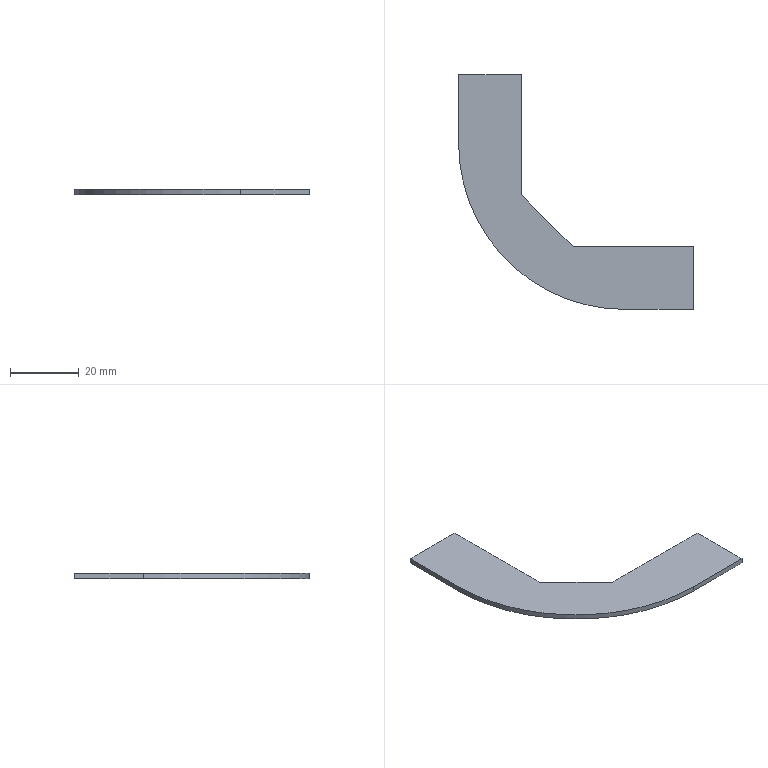Part | SolidWorks | features MirrorStock 1 | 1 solid | 10 faces | box 68.3 x 68.3 x 1.5 mm | volume 2665 mm3 | plane 9 | cylinder 1 | commonest cylinder face diameters 96.6 x1
STEP:
#1=CARTESIAN_POINT('',(46.96,45.489,0.));
#2=VERTEX_POINT('',#1);
#3=CARTESIAN_POINT('',(28.66,45.489,0.));
#4=VERTEX_POINT('',#3);
#5=CARTESIAN_POINT('',(28.66,45.489,0.));
#6=DIRECTION('',(-1.,0.,0.));
#7=VECTOR('',#6,1000.);
#8=LINE('',#5,#7);
#9=EDGE_CURVE('',#2,#4,#8,.T.);
#10=ORIENTED_EDGE('',*,*,#9,.F.);
#11=CARTESIAN_POINT('',(46.96,45.489,-1.5));
#12=VERTEX_POINT('',#11);
#13=CARTESIAN_POINT('',(46.96,45.489,-1.5));
#14=DIRECTION('',(0.,0.,1.));
#15=VECTOR('',#14,1000.);
#16=LINE('',#13,#15);
#17=EDGE_CURVE('',#12,#2,#16,.T.);
#18=ORIENTED_EDGE('',*,*,#17,.F.);
#19=CARTESIAN_POINT('',(28.66,45.489,-1.5));
#20=VERTEX_POINT('',#19);
#21=CARTESIAN_POINT('',(28.66,45.489,-1.5));
#22=DIRECTION('',(-1.,0.,0.));
#23=VECTOR('',#22,1000.);
#24=LINE('',#21,#23);
#25=EDGE_CURVE('',#12,#20,#24,.T.);
#26=ORIENTED_EDGE('',*,*,#25,.T.);
#27=CARTESIAN_POINT('',(28.66,45.489,-1.5));
#28=DIRECTION('',(0.,0.,1.));
#29=VECTOR('',#28,1000.);
#30=LINE('',#27,#29);
#31=EDGE_CURVE('',#20,#4,#30,.T.);
#32=ORIENTED_EDGE('',*,*,#31,.T.);
#33=EDGE_LOOP('',(#10,#18,#26,#32));
#34=FACE_OUTER_BOUND('',#33,.T.);
#35=CARTESIAN_POINT('',(28.66,45.489,-1.5));
#36=DIRECTION('',(0.,-1.,0.));
#37=DIRECTION('',(0.,0.,1.));
#38=AXIS2_PLACEMENT_3D('',#35,#36,#37);
#39=PLANE('',#38);
#40=ADVANCED_FACE('',(#34),#39,.F.);
#41=CARTESIAN_POINT('',(28.66,25.489,0.));
#42=VERTEX_POINT('',#41);
#43=CARTESIAN_POINT('',(28.66,45.489,0.));
#44=DIRECTION('',(0.,-1.,0.));
#45=VECTOR('',#44,1000.);
#46=LINE('',#43,#45);
#47=EDGE_CURVE('',#4,#42,#46,.T.);
#48=ORIENTED_EDGE('',*,*,#47,.F.);
#49=ORIENTED_EDGE('',*,*,#31,.F.);
#50=CARTESIAN_POINT('',(28.66,25.489,-1.5));
#51=VERTEX_POINT('',#50);
#52=CARTESIAN_POINT('',(28.66,45.489,-1.5));
#53=DIRECTION('',(0.,-1.,0.));
#54=VECTOR('',#53,1000.);
#55=LINE('',#52,#54);
#56=EDGE_CURVE('',#20,#51,#55,.T.);
#57=ORIENTED_EDGE('',*,*,#56,.T.);
#58=CARTESIAN_POINT('',(28.66,25.489,-1.5));
#59=DIRECTION('',(0.,0.,1.));
#60=VECTOR('',#59,1000.);
#61=LINE('',#58,#60);
#62=EDGE_CURVE('',#51,#42,#61,.T.);
#63=ORIENTED_EDGE('',*,*,#62,.T.);
#64=EDGE_LOOP('',(#48,#49,#57,#63));
#65=FACE_OUTER_BOUND('',#64,.T.);
#66=CARTESIAN_POINT('',(28.66,45.489,-1.5));
#67=DIRECTION('',(1.,0.,0.));
#68=DIRECTION('',(0.,0.,1.));
#69=AXIS2_PLACEMENT_3D('',#66,#67,#68);
#70=PLANE('',#69);
#71=ADVANCED_FACE('',(#65),#70,.F.);
#72=CARTESIAN_POINT('',(76.96,-22.811,0.));
#73=VERTEX_POINT('',#72);
#74=CARTESIAN_POINT('',(76.96,25.489,0.));
#75=DIRECTION('',(0.,0.,1.));
#76=DIRECTION('',(-1.,0.,0.));
#77=AXIS2_PLACEMENT_3D('',#74,#75,#76);
#78=CIRCLE('',#77,48.3);
#79=EDGE_CURVE('',#42,#73,#78,.T.);
#80=ORIENTED_EDGE('',*,*,#79,.F.);
#81=ORIENTED_EDGE('',*,*,#62,.F.);
#82=CARTESIAN_POINT('',(76.96,-22.811,-1.5));
#83=VERTEX_POINT('',#82);
#84=CARTESIAN_POINT('',(76.96,25.489,-1.5));
#85=DIRECTION('',(0.,0.,1.));
#86=DIRECTION('',(-1.,0.,0.));
#87=AXIS2_PLACEMENT_3D('',#84,#85,#86);
#88=CIRCLE('',#87,48.3);
#89=EDGE_CURVE('',#51,#83,#88,.T.);
#90=ORIENTED_EDGE('',*,*,#89,.T.);
#91=CARTESIAN_POINT('',(76.96,-22.811,-1.5));
#92=DIRECTION('',(0.,0.,1.));
#93=VECTOR('',#92,1000.);
#94=LINE('',#91,#93);
#95=EDGE_CURVE('',#83,#73,#94,.T.);
#96=ORIENTED_EDGE('',*,*,#95,.T.);
#97=EDGE_LOOP('',(#80,#81,#90,#96));
#98=FACE_OUTER_BOUND('',#97,.T.);
#99=CARTESIAN_POINT('',(76.96,25.489,-1.5));
#100=DIRECTION('',(0.,0.,1.));
#101=DIRECTION('',(-1.,0.,0.));
#102=AXIS2_PLACEMENT_3D('',#99,#100,#101);
#103=CYLINDRICAL_SURFACE('',#102,48.3);
#104=ADVANCED_FACE('',(#98),#103,.T.);
#105=CARTESIAN_POINT('',(96.96,-22.811,0.));
#106=VERTEX_POINT('',#105);
#107=CARTESIAN_POINT('',(76.96,-22.811,0.));
#108=DIRECTION('',(1.,0.,0.));
#109=VECTOR('',#108,1000.);
#110=LINE('',#107,#109);
#111=EDGE_CURVE('',#73,#106,#110,.T.);
#112=ORIENTED_EDGE('',*,*,#111,.F.);
#113=ORIENTED_EDGE('',*,*,#95,.F.);
#114=CARTESIAN_POINT('',(96.96,-22.811,-1.5));
#115=VERTEX_POINT('',#114);
#116=CARTESIAN_POINT('',(76.96,-22.811,-1.5));
#117=DIRECTION('',(1.,0.,0.));
#118=VECTOR('',#117,1000.);
#119=LINE('',#116,#118);
#120=EDGE_CURVE('',#83,#115,#119,.T.);
#121=ORIENTED_EDGE('',*,*,#120,.T.);
#122=CARTESIAN_POINT('',(96.96,-22.811,-1.5));
#123=DIRECTION('',(0.,0.,1.));
#124=VECTOR('',#123,1000.);
#125=LINE('',#122,#124);
#126=EDGE_CURVE('',#115,#106,#125,.T.);
#127=ORIENTED_EDGE('',*,*,#126,.T.);
#128=EDGE_LOOP('',(#112,#113,#121,#127));
#129=FACE_OUTER_BOUND('',#128,.T.);
#130=CARTESIAN_POINT('',(76.96,-22.811,-1.5));
#131=DIRECTION('',(0.,1.,0.));
#132=DIRECTION('',(0.,0.,-1.));
#133=AXIS2_PLACEMENT_3D('',#130,#131,#132);
#134=PLANE('',#133);
#135=ADVANCED_FACE('',(#129),#134,.F.);
#136=CARTESIAN_POINT('',(96.96,-4.511,0.));
#137=VERTEX_POINT('',#136);
#138=CARTESIAN_POINT('',(96.96,-4.511,0.));
#139=DIRECTION('',(0.,1.,0.));
#140=VECTOR('',#139,1000.);
#141=LINE('',#138,#140);
#142=EDGE_CURVE('',#106,#137,#141,.T.);
#143=ORIENTED_EDGE('',*,*,#142,.F.);
#144=ORIENTED_EDGE('',*,*,#126,.F.);
#145=CARTESIAN_POINT('',(96.96,-4.511,-1.5));
#146=VERTEX_POINT('',#145);
#147=CARTESIAN_POINT('',(96.96,-4.511,-1.5));
#148=DIRECTION('',(0.,1.,0.));
#149=VECTOR('',#148,1000.);
#150=LINE('',#147,#149);
#151=EDGE_CURVE('',#115,#146,#150,.T.);
#152=ORIENTED_EDGE('',*,*,#151,.T.);
#153=CARTESIAN_POINT('',(96.96,-4.511,-1.5));
#154=DIRECTION('',(0.,0.,1.));
#155=VECTOR('',#154,1000.);
#156=LINE('',#153,#155);
#157=EDGE_CURVE('',#146,#137,#156,.T.);
#158=ORIENTED_EDGE('',*,*,#157,.T.);
#159=EDGE_LOOP('',(#143,#144,#152,#158));
#160=FACE_OUTER_BOUND('',#159,.T.);
#161=CARTESIAN_POINT('',(96.96,-4.511,-1.5));
#162=DIRECTION('',(-1.,0.,0.));
#163=DIRECTION('',(0.,0.,-1.));
#164=AXIS2_PLACEMENT_3D('',#161,#162,#163);
#165=PLANE('',#164);
#166=ADVANCED_FACE('',(#160),#165,.F.);
#167=CARTESIAN_POINT('',(61.96,-4.511,0.));
#168=VERTEX_POINT('',#167);
#169=CARTESIAN_POINT('',(61.96,-4.511,0.));
#170=DIRECTION('',(-1.,0.,0.));
#171=VECTOR('',#170,1000.);
#172=LINE('',#169,#171);
#173=EDGE_CURVE('',#137,#168,#172,.T.);
#174=ORIENTED_EDGE('',*,*,#173,.F.);
#175=ORIENTED_EDGE('',*,*,#157,.F.);
#176=CARTESIAN_POINT('',(61.96,-4.511,-1.5));
#177=VERTEX_POINT('',#176);
#178=CARTESIAN_POINT('',(61.96,-4.511,-1.5));
#179=DIRECTION('',(-1.,0.,0.));
#180=VECTOR('',#179,1000.);
#181=LINE('',#178,#180);
#182=EDGE_CURVE('',#146,#177,#181,.T.);
#183=ORIENTED_EDGE('',*,*,#182,.T.);
#184=CARTESIAN_POINT('',(61.96,-4.511,-1.5));
#185=DIRECTION('',(0.,0.,1.));
#186=VECTOR('',#185,1000.);
#187=LINE('',#184,#186);
#188=EDGE_CURVE('',#177,#168,#187,.T.);
#189=ORIENTED_EDGE('',*,*,#188,.T.);
#190=EDGE_LOOP('',(#174,#175,#183,#189));
#191=FACE_OUTER_BOUND('',#190,.T.);
#192=CARTESIAN_POINT('',(61.96,-4.511,-1.5));
#193=DIRECTION('',(0.,-1.,0.));
#194=DIRECTION('',(1.,0.,0.));
#195=AXIS2_PLACEMENT_3D('',#192,#193,#194);
#196=PLANE('',#195);
#197=ADVANCED_FACE('',(#191),#196,.F.);
#198=CARTESIAN_POINT('',(46.96,10.489,0.));
#199=VERTEX_POINT('',#198);
#200=CARTESIAN_POINT('',(46.96,10.489,0.));
#201=DIRECTION('',(-0.7071,0.7071,0.));
#202=VECTOR('',#201,1000.);
#203=LINE('',#200,#202);
#204=EDGE_CURVE('',#168,#199,#203,.T.);
#205=ORIENTED_EDGE('',*,*,#204,.F.);
#206=ORIENTED_EDGE('',*,*,#188,.F.);
#207=CARTESIAN_POINT('',(46.96,10.489,-1.5));
#208=VERTEX_POINT('',#207);
#209=CARTESIAN_POINT('',(46.96,10.489,-1.5));
#210=DIRECTION('',(-0.7071,0.7071,0.));
#211=VECTOR('',#210,1000.);
#212=LINE('',#209,#211);
#213=EDGE_CURVE('',#177,#208,#212,.T.);
#214=ORIENTED_EDGE('',*,*,#213,.T.);
#215=CARTESIAN_POINT('',(46.96,10.489,-1.5));
#216=DIRECTION('',(0.,0.,1.));
#217=VECTOR('',#216,1000.);
#218=LINE('',#215,#217);
#219=EDGE_CURVE('',#208,#199,#218,.T.);
#220=ORIENTED_EDGE('',*,*,#219,.T.);
#221=EDGE_LOOP('',(#205,#206,#214,#220));
#222=FACE_OUTER_BOUND('',#221,.T.);
#223=CARTESIAN_POINT('',(46.96,10.489,-1.5));
#224=DIRECTION('',(-0.7071,-0.7071,0.));
#225=DIRECTION('',(0.7071,-0.7071,0.));
#226=AXIS2_PLACEMENT_3D('',#223,#224,#225);
#227=PLANE('',#226);
#228=ADVANCED_FACE('',(#222),#227,.F.);
#229=CARTESIAN_POINT('',(46.96,45.489,0.));
#230=DIRECTION('',(0.,1.,0.));
#231=VECTOR('',#230,1000.);
#232=LINE('',#229,#231);
#233=EDGE_CURVE('',#199,#2,#232,.T.);
#234=ORIENTED_EDGE('',*,*,#233,.F.);
#235=ORIENTED_EDGE('',*,*,#219,.F.);
#236=CARTESIAN_POINT('',(46.96,45.489,-1.5));
#237=DIRECTION('',(0.,1.,0.));
#238=VECTOR('',#237,1000.);
#239=LINE('',#236,#238);
#240=EDGE_CURVE('',#208,#12,#239,.T.);
#241=ORIENTED_EDGE('',*,*,#240,.T.);
#242=ORIENTED_EDGE('',*,*,#17,.T.);
#243=EDGE_LOOP('',(#234,#235,#241,#242));
#244=FACE_OUTER_BOUND('',#243,.T.);
#245=CARTESIAN_POINT('',(46.96,45.489,-1.5));
#246=DIRECTION('',(-1.,0.,0.));
#247=DIRECTION('',(0.,0.,-1.));
#248=AXIS2_PLACEMENT_3D('',#245,#246,#247);
#249=PLANE('',#248);
#250=ADVANCED_FACE('',(#244),#249,.F.);
#251=ORIENTED_EDGE('',*,*,#25,.F.);
#252=ORIENTED_EDGE('',*,*,#240,.F.);
#253=ORIENTED_EDGE('',*,*,#213,.F.);
#254=ORIENTED_EDGE('',*,*,#182,.F.);
#255=ORIENTED_EDGE('',*,*,#151,.F.);
#256=ORIENTED_EDGE('',*,*,#120,.F.);
#257=ORIENTED_EDGE('',*,*,#89,.F.);
#258=ORIENTED_EDGE('',*,*,#56,.F.);
#259=EDGE_LOOP('',(#251,#252,#253,#254,#255,#256,#257,#258));
#260=FACE_OUTER_BOUND('',#259,.T.);
#261=CARTESIAN_POINT('',(76.96,25.489,-1.5));
#262=DIRECTION('',(0.,0.,1.));
#263=DIRECTION('',(-1.,0.,0.));
#264=AXIS2_PLACEMENT_3D('',#261,#262,#263);
#265=PLANE('',#264);
#266=ADVANCED_FACE('',(#260),#265,.F.);
#267=ORIENTED_EDGE('',*,*,#9,.T.);
#268=ORIENTED_EDGE('',*,*,#47,.T.);
#269=ORIENTED_EDGE('',*,*,#79,.T.);
#270=ORIENTED_EDGE('',*,*,#111,.T.);
#271=ORIENTED_EDGE('',*,*,#142,.T.);
#272=ORIENTED_EDGE('',*,*,#173,.T.);
#273=ORIENTED_EDGE('',*,*,#204,.T.);
#274=ORIENTED_EDGE('',*,*,#233,.T.);
#275=EDGE_LOOP('',(#267,#268,#269,#270,#271,#272,#273,#274));
#276=FACE_OUTER_BOUND('',#275,.T.);
#277=CARTESIAN_POINT('',(76.96,25.489,0.));
#278=DIRECTION('',(0.,0.,1.));
#279=DIRECTION('',(-1.,0.,0.));
#280=AXIS2_PLACEMENT_3D('',#277,#278,#279);
#281=PLANE('',#280);
#282=ADVANCED_FACE('',(#276),#281,.T.);
#283=CLOSED_SHELL('',(#40,#71,#104,#135,#166,#197,#228,#250,#266,#282));
#284=MANIFOLD_SOLID_BREP('',#283);
#285=CARTESIAN_POINT('',(0.,0.,0.));
#286=DIRECTION('',(0.,0.,1.));
#287=DIRECTION('',(1.,0.,0.));
#288=AXIS2_PLACEMENT_3D('',#285,#286,#287);
#289=(LENGTH_UNIT()NAMED_UNIT(*)SI_UNIT(.MILLI.,.METRE.));
#290=UNCERTAINTY_MEASURE_WITH_UNIT(LENGTH_MEASURE(0.00001),#289,'','');
#291=(NAMED_UNIT(*)PLANE_ANGLE_UNIT()SI_UNIT($,.RADIAN.));
#292=(NAMED_UNIT(*)SI_UNIT($,.STERADIAN.)SOLID_ANGLE_UNIT());
#293=(GEOMETRIC_REPRESENTATION_CONTEXT(3)GLOBAL_UNCERTAINTY_ASSIGNED_CONTEXT((#290))GLOBAL_UNIT_ASSIGNED_CONTEXT((#289,#291,#292))REPRESENTATION_CONTEXT('',''));
#294=ADVANCED_BREP_SHAPE_REPRESENTATION('',(#284,#288),#293);